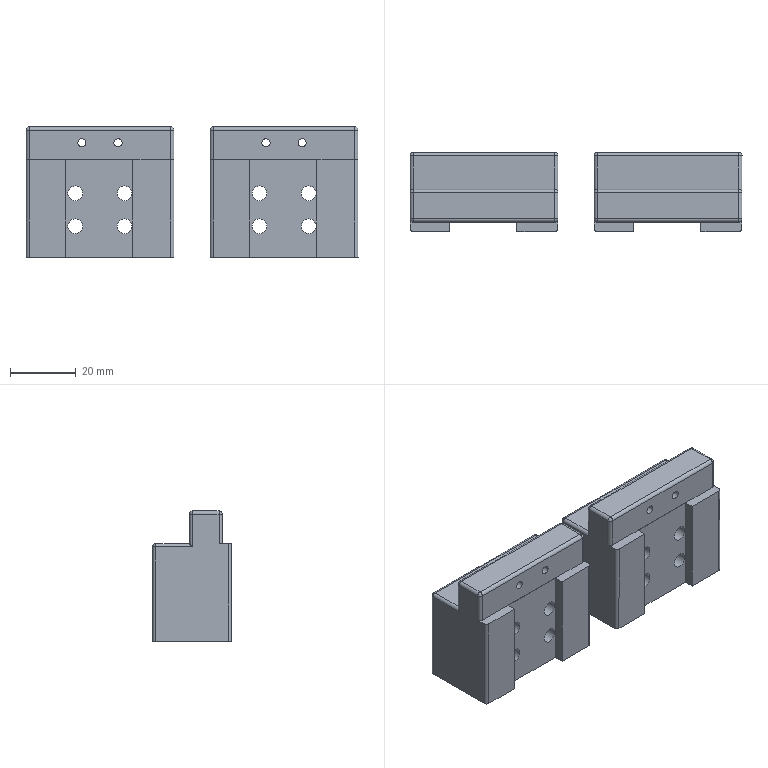CAM job | NX | 3+2 milling, drilling | part box 101.001 x 24.001 x 39.667 mm | stock box 106.001 x 30.002 x 40.668 mm
Tools:
number,name,description,diameter,corner_radius,flute_length,length,flutes
4,D4,平底铣刀-粗,4.0,0.0,50.0,75.0,2
9,D10,平底铣刀-粗,10.0,0.0,50.0,75.0,2
18,D4-J,平底铣刀-精,4.0,0.0,50.0,75.0,2
7,D6-J,平底铣刀-精,6.0,0.0,50.0,75.0,2
10,D10-J,平底铣刀-精,10.0,0.0,50.0,75.0,2
17,D4R0.5,圆鼻刀-粗,4.0,0.5,50.0,75.0,2
1,D80R0.8_FACEMILL,圆鼻刀-粗,80.0,0.8,50.0,75.0,2
2,D6_CHAMFERMILL,倒角刀,6.0,0.0,3.0,75.0,2
20,M3X0.5,丝锥,2.5,0.0,35.0,50.0,2
21,M4X0.7,丝锥,3.3,0.0,35.0,50.0,2
12,ZT2.5,钻头,2.5,0.0,35.0,50.0,2
11,ZT4.5,钻头,4.5,0.0,35.0,50.0,2
19,DRILL3.3,Twist Drill 3.3 mm,3.3,0.0,35.0,35.008,2
18,TXD11H1.5,Milling Tool-T Cutter,11.0,,1.5,50.0,4
Operations:
program,operation,operation_type,tool,method,geometry_group,spindle_rpm,surface_speed,feed_per_tooth,feed_cut,feed_plunge,cut_length_mm,path_length_mm,cut_time_min,machine_time_min
C,FLOORWALL_LAYERROUGH-MID_COPY_1,VolumeBased25DMillingOperation,D10,LAYERROUGH-DEPTHK-STEPG,W-C,8000.0,251.327,0.125,2000.0,100.0,464.056,610.2,0.232,0.2466
C,ZLEVEL_FINISH-MID_COPY_2_COPY,ZLevelMilling,D10,SIDEFINISH-DEPTHK-STEPG,W-C,8000.0,251.32,0.0625,1000.0,100.0,54.565,68.765,0.0546,0.056
C,SPOT-DEPTH0.8_2,Operation,D6_CHAMFERMILL,NONE,W-C,8000.0,150.796,0.0312,500.0,90.0,5.4,93.81,0.0108,0.0196
C,BLINDFLAT-M3TAPDRILL,Operation,ZT2.5,NONE,W-C,3000.0,23.562,0.02,120.0,90.0,11.0,71,0.0917,0.0977
C,BLINDFLAT-M4TAPDRILL,Operation,DRILL3.3,NONE,W-C,3000.0,31.102,0.0167,100.0,90.0,36.0,147.015,0.36,0.3711
C,DRILLCHAMFER_3,Operation,D6_CHAMFERMILL,METHOD,W-C,8000.0,150.796,0.0312,500.0,0.0,4.75,58.5,0.0095,0.0149
C,DRILLCHAMFER_4,Operation,D6_CHAMFERMILL,METHOD,W-C,8000.0,150.796,0.0312,500.0,0.0,10.4,97.932,0.0208,0.0296
C,BLINDFLAT-TAPM3,Operation,M3X0.5,METHOD,W-C,800.0,6.283,0.0003,0.5,90.0,7.5,64,15.0,15.006
C,BLINDFLAT-TAPM4,Operation,M4X0.7,METHOD,W-C,800.0,8.294,0.0004,0.7,90.0,30.0,135.015,42.857,42.868
C,PLANARDEBURR6X45L_COPY_1,SurfaceContour,D6_CHAMFERMILL,WALLCHAMFER-DEPTH0-STEPG,W-C,6500.0,122.519,0.1154,1500.0,100.0,200.124,353.432,0.1334,0.1487
C,FLOORWALL_FINISHSIDE-MID-SELBOTTOM_COPY,VolumeBased25DMillingOperation,D10-J,SIDEFINISH-DEPTHK-STEPG,W-C,8000.0,251.32,0.0625,1000.0,100.0,55.46,82.46,0.0555,0.0582
C,ZLEVEL_FINISH-MID_COPY_2,ZLevelMilling,D10-J,SIDEFINISH-DEPTHK-STEPG,W-C,8000.0,251.32,0.0625,1000.0,100.0,54.57,68.57,0.0546,0.056
C,PLANAR_FINISHSIDE-MID_COPY_2,PlanarMilling,TXD11H1.5,SIDEFINISH-DEPTHK-STEPG,W-C,8000.0,251.327,0.0312,500.0,100.0,61.187,108.186,0.1224,0.1271
C,PLANAR_FINISHSIDE-MID_COPY_2_COPY,PlanarMilling,TXD11H1.5,SIDEFINISH-DEPTHK-STEPG,W-C,8000.0,251.327,0.0312,500.0,100.0,61.873,108.873,0.1237,0.1284
B,AUTOFACEMILL_ROUGH1_COPY,FaceMilling,D80R0.8_FACEMILL,LAYERROUGH-DEPTHK-STEPG,W-B,4500.0,890.615,0.3333,3000.0,100.0,2299.016,4414.648,0.7663,0.9779
B,AUTOFACEMILL_FINISH1_COPY,FaceMilling,D80R0.8_FACEMILL,SIDEFINISH-DEPTHK-STEPG,W-B,4500.0,890.615,0.1111,1000.0,100.0,209.001,245.001,0.209,0.2126
B,CAVITY_ROUGH-MID_COPY,CavityMilling,D10,LAYERROUGH-DEPTHK-STEPG,W-B,8000.0,251.32,0.25,4000.0,100.0,3002.639,3508.923,0.7507,0.8102
B,ZLEVEL_FINISHRECIPWALL_COPY_COPY_1,ZLevelMilling,D4R0.5,ZLEVELWALL-DEPTHK-STEPG,W-B,8000.0,100.531,0.3125,5000.0,100.0,2826.052,3102.019,0.5652,0.5928
B,DRILLCHAMFER_2,Operation,D6_CHAMFERMILL,METHOD,W-B,8000.0,150.796,0.0625,1000.0,0.0,19.0,160.472,0.019,0.0331
B,PLANARDEBURR6X45L_COPY,SurfaceContour,D6_CHAMFERMILL,WALLCHAMFER-DEPTH0-STEPG,W-B,6500.0,122.519,0.1154,1500.0,100.0,296.939,860.045,0.198,0.2543
B,PLANAR_C0.3CLOSEDCONTOURCHAMFER6X45L_COPY,PlanarMilling,D6_CHAMFERMILL,WALLCHAMFER-DEPTH0-STEPG,W-B,7000.0,131.0,0.1071,1500.0,100.0,101.24,137.243,0.0675,0.0711
B,CAVITY_FINISHBOTTOM-MID_COPY_1,CavityMilling,D4-J,SIDEFINISH-DEPTHK-STEPG,W-B,8000.0,100.528,0.05,800.0,100.0,1403.468,1836.931,1.754,1.798
B,ZLEVEL_FINISH-MID_COPY_1,ZLevelMilling,D4-J,SIDEFINISH-DEPTHK-STEPG,W-B,8000.0,100.528,0.05,800.0,100.0,238.249,669.864,0.2978,0.341
B,ZLEVEL_FINISHRECIPWALL_COPY_COPY_1_COPY,ZLevelMilling,D4-J,ZLEVELWALL-DEPTHK-STEPG,W-B,8000.0,100.531,0.3125,5000.0,100.0,12873.079,13053.36,2.575,2.593
B,PLANAR_FINISHSIDE-MID_COPY_1,PlanarMilling,D4-J,SIDEFINISH-DEPTHK-STEPG,W-B,8000.0,100.528,0.05,800.0,100.0,106.8,249.937,0.1335,0.1478
A,FACEMILL_TOPFACE,FaceMilling,D80R0.8_FACEMILL,SIDEFINISH-DEPTHK-STEPG,W-A,4000.0,1005.31,0.125,1000.0,100.0,195.001,231.001,0.195,0.1986
A,PROFILE_ROUGH_2,VolumeBased25DMillingOperation,D10,METHOD,W-A,8000.0,251.327,0.3125,5000.0,80.0,13641.373,13911.804,2.728,2.755
A,FLOORWALL_LAYERROUGH-MID_COPY,VolumeBased25DMillingOperation,D10,LAYERROUGH-DEPTHK-STEPG,W-A,8000.0,251.32,0.25,4000.0,100.0,5343.675,5401.064,1.336,1.342
A,SPOT-DEPTH0.8,Operation,D6_CHAMFERMILL,NONE,W-A,8000.0,150.796,0.0312,500.0,90.0,21.6,288.483,0.0432,0.0699
A,THRU-M3TAPDRILL,Operation,ZT2.5,NONE,W-A,3000.0,23.562,0.05,300.0,90.0,66.836,266.292,0.2228,0.2427
A,CBORE-DRILL0SEG,Operation,ZT4.5,NONE,W-A,2800.0,39.584,0.0179,100.0,90.0,203.619,565.517,2.036,2.072
A,HOLEROUGH_D4_1,CylinderMilling,D4,NONE,W-A,8000.0,100.531,0.075,1200.0,100.0,5079.209,5626.221,4.233,4.287
A,ZLEVEL_FINISHRECIPWALL_COPY,ZLevelMilling,D4R0.5,ZLEVELWALL-DEPTHK-STEPG,W-A,8000.0,100.531,0.3125,5000.0,100.0,5313.997,5415.394,1.063,1.073
A,BODYONLY,SurfaceContour,D6_CHAMFERMILL,METHOD,W-A,8000.0,150.796,0.1875,3000.0,100.0,92.477,393.299,0.0308,0.0609
A,DRILLCHAMFER_1,Operation,D6_CHAMFERMILL,METHOD,W-A,8000.0,150.796,0.0312,500.0,0.0,19.0,177.422,0.038,0.0538
A,MILL_CHAMFER_1,PlanarMilling,D6_CHAMFERMILL,NONE,W-A,8000.0,150.796,0.0312,500.0,100.0,233.309,664.929,0.4666,0.5098
A,HOLEFINISH_D4_1,CylinderMilling,D4-J,FINISH-STEPDEPTHOFF,W-A,8000.0,100.531,0.0312,500.0,100.0,485.745,1032.756,0.9715,1.026
A,THRU-TAPM3,Operation,M3X0.5,METHOD,W-A,800.0,6.283,0.0003,0.5,90.0,55.831,244.283,111.662,111.681
A,CAVITY_FINISHBOTTOM-MID_COPY,CavityMilling,D6-J,SIDEFINISH-DEPTHK-STEPG,W-A,8000.0,150.792,0.0625,1000.0,100.0,484.483,797.345,0.4845,0.5158
A,ZLEVEL_FINISH-MID_COPY,ZLevelMilling,D6-J,SIDEFINISH-DEPTHK-STEPG,W-A,8000.0,251.32,0.0625,1000.0,100.0,121.604,293.839,0.1216,0.1388
A,ZLEVEL_FINISHRECIPWALL_COPY_COPY,ZLevelMilling,D6-J,ZLEVELWALL-DEPTHK-STEPG,W-A,8000.0,100.531,0.3125,5000.0,100.0,13592.272,13739.979,2.719,2.733
A,PROFILE_SEMI_2,VolumeBased25DMillingOperation,D6-J,METHOD,W-A,8000.0,251.327,0.0625,1000.0,100.0,769.101,1135.652,0.7691,0.8058